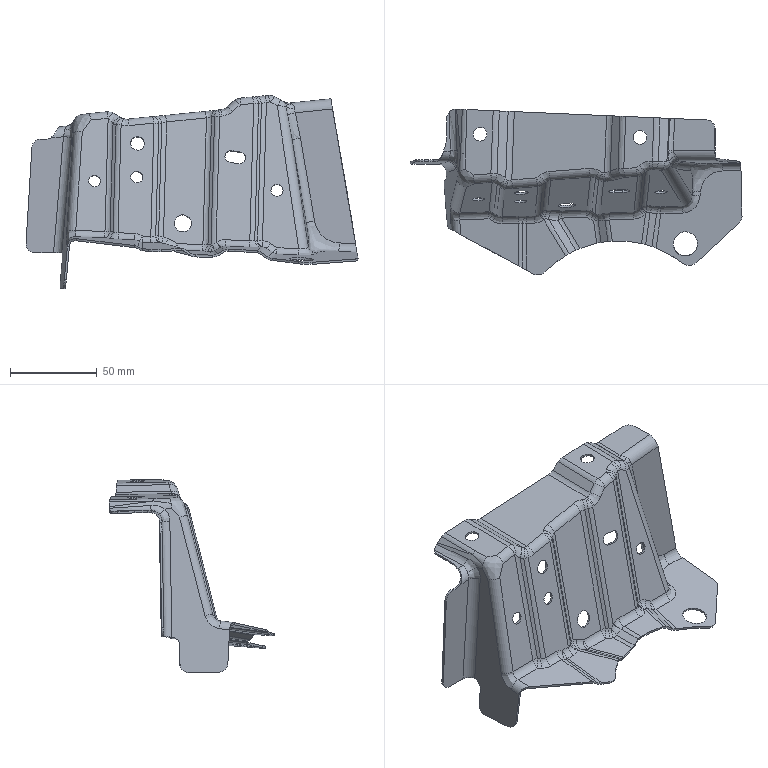Part | 1 solid | 366 faces | box 190.934 x 95.254 x 111.136 mm | volume 31856 mm3 | spline 165 | cylinder 132 | plane 43 | sphere 24 | other 2 | commonest cylinder face diameters 10 x49 12.4 x24 7.6 x23 12 x9 7 x8 8 x6